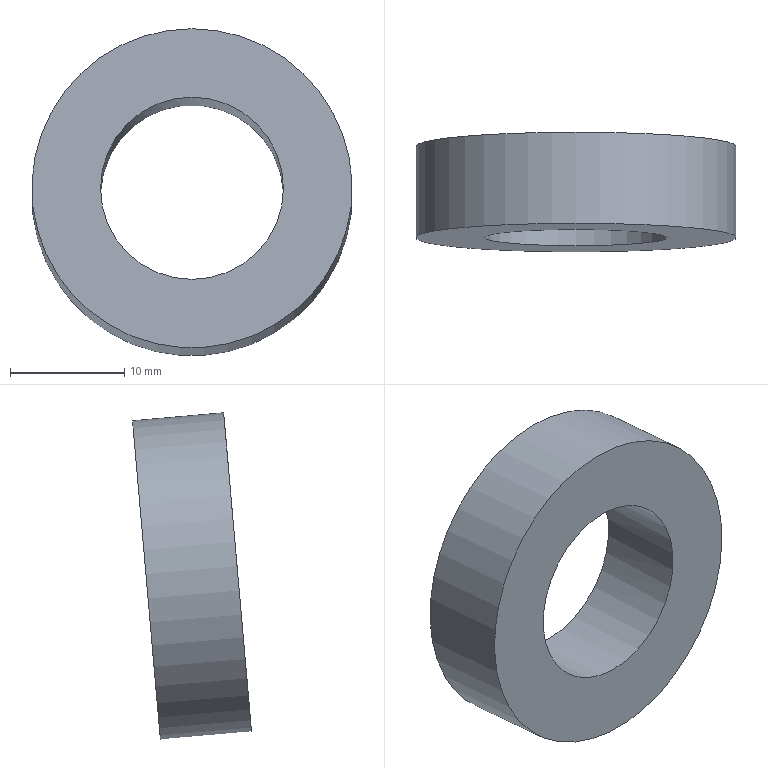Part | NX | features solid 2 | 1 solid | 4 faces | box 28 x 10.41 x 28.591 mm | volume 3318 mm3 | cylinder 2 | plane 2 | commonest cylinder face diameters 16 x1 28 x1
STEP:
#1=CARTESIAN_POINT('',(-120.452,-55.988,-22.095));
#2=VERTEX_POINT('',#1);
#3=CARTESIAN_POINT('',(-120.452,-57.209,-36.042));
#4=DIRECTION('',(0.,0.9962,-0.08716));
#5=DIRECTION('',(0.,0.08716,0.9962));
#6=AXIS2_PLACEMENT_3D('',#3,#4,#5);
#7=CIRCLE('',#6,14.);
#8=EDGE_CURVE('',#2,#2,#7,.F.);
#9=ORIENTED_EDGE('',*,*,#8,.T.);
#10=EDGE_LOOP('',(#9));
#11=FACE_BOUND('',#10,.T.);
#12=CARTESIAN_POINT('',(-120.452,-63.958,-21.398));
#13=VERTEX_POINT('',#12);
#14=CARTESIAN_POINT('',(-120.452,-65.178,-35.345));
#15=DIRECTION('',(0.,0.9962,-0.08716));
#16=DIRECTION('',(0.,0.08716,0.9962));
#17=AXIS2_PLACEMENT_3D('',#14,#15,#16);
#18=CIRCLE('',#17,14.);
#19=EDGE_CURVE('',#13,#13,#18,.F.);
#20=ORIENTED_EDGE('',*,*,#19,.F.);
#21=EDGE_LOOP('',(#20));
#22=FACE_BOUND('',#21,.T.);
#23=CARTESIAN_POINT('',(-120.452,-58.205,-35.955));
#24=DIRECTION('',(0.,-0.9962,0.08716));
#25=DIRECTION('',(0.,-0.08716,-0.9962));
#26=AXIS2_PLACEMENT_3D('',#23,#24,#25);
#27=CYLINDRICAL_SURFACE('',#26,14.);
#28=ADVANCED_FACE('',(#11,#22),#27,.T.);
#29=CARTESIAN_POINT('',(-120.452,-57.906,-44.012));
#30=VERTEX_POINT('',#29);
#31=CARTESIAN_POINT('',(-120.452,-57.209,-36.042));
#32=DIRECTION('',(0.,-0.9962,0.08716));
#33=DIRECTION('',(0.,-0.08716,-0.9962));
#34=AXIS2_PLACEMENT_3D('',#31,#32,#33);
#35=CIRCLE('',#34,8.);
#36=EDGE_CURVE('',#30,#30,#35,.T.);
#37=ORIENTED_EDGE('',*,*,#36,.T.);
#38=EDGE_LOOP('',(#37));
#39=FACE_BOUND('',#38,.T.);
#40=ORIENTED_EDGE('',*,*,#8,.F.);
#41=EDGE_LOOP('',(#40));
#42=FACE_BOUND('',#41,.T.);
#43=CARTESIAN_POINT('',(-120.452,-57.209,-36.042));
#44=DIRECTION('',(0.,0.9962,-0.08716));
#45=DIRECTION('',(-1.,0.,0.));
#46=AXIS2_PLACEMENT_3D('',#43,#44,#45);
#47=PLANE('',#46);
#48=ADVANCED_FACE('',(#39,#42),#47,.T.);
#49=CARTESIAN_POINT('',(-120.452,-64.481,-27.375));
#50=VERTEX_POINT('',#49);
#51=CARTESIAN_POINT('',(-120.452,-65.178,-35.345));
#52=DIRECTION('',(0.,0.9962,-0.08716));
#53=DIRECTION('',(0.,0.08716,0.9962));
#54=AXIS2_PLACEMENT_3D('',#51,#52,#53);
#55=CIRCLE('',#54,8.);
#56=EDGE_CURVE('',#50,#50,#55,.T.);
#57=ORIENTED_EDGE('',*,*,#56,.T.);
#58=EDGE_LOOP('',(#57));
#59=FACE_BOUND('',#58,.T.);
#60=ORIENTED_EDGE('',*,*,#19,.T.);
#61=EDGE_LOOP('',(#60));
#62=FACE_BOUND('',#61,.T.);
#63=CARTESIAN_POINT('',(-120.452,-65.178,-35.345));
#64=DIRECTION('',(0.,0.9962,-0.08716));
#65=DIRECTION('',(-1.,0.,0.));
#66=AXIS2_PLACEMENT_3D('',#63,#64,#65);
#67=PLANE('',#66);
#68=ADVANCED_FACE('',(#59,#62),#67,.F.);
#69=ORIENTED_EDGE('',*,*,#36,.F.);
#70=EDGE_LOOP('',(#69));
#71=FACE_BOUND('',#70,.T.);
#72=ORIENTED_EDGE('',*,*,#56,.F.);
#73=EDGE_LOOP('',(#72));
#74=FACE_BOUND('',#73,.T.);
#75=CARTESIAN_POINT('',(-120.452,-57.209,-36.042));
#76=DIRECTION('',(0.,-0.9962,0.08716));
#77=DIRECTION('',(0.,-0.08716,-0.9962));
#78=AXIS2_PLACEMENT_3D('',#75,#76,#77);
#79=CYLINDRICAL_SURFACE('',#78,8.);
#80=ADVANCED_FACE('',(#71,#74),#79,.F.);
#81=CLOSED_SHELL('',(#28,#48,#68,#80));
#82=MANIFOLD_SOLID_BREP('',#81);
#83=(LENGTH_UNIT()NAMED_UNIT(*)SI_UNIT(.MILLI.,.METRE.));
#84=UNCERTAINTY_MEASURE_WITH_UNIT(LENGTH_MEASURE(0.00001),#83,'','');
#85=(NAMED_UNIT(*)PLANE_ANGLE_UNIT()SI_UNIT($,.RADIAN.));
#86=(NAMED_UNIT(*)SI_UNIT($,.STERADIAN.)SOLID_ANGLE_UNIT());
#87=(GEOMETRIC_REPRESENTATION_CONTEXT(3)GLOBAL_UNCERTAINTY_ASSIGNED_CONTEXT((#84))GLOBAL_UNIT_ASSIGNED_CONTEXT((#83,#85,#86))REPRESENTATION_CONTEXT('',''));
#88=ADVANCED_BREP_SHAPE_REPRESENTATION('',(#82),#87);